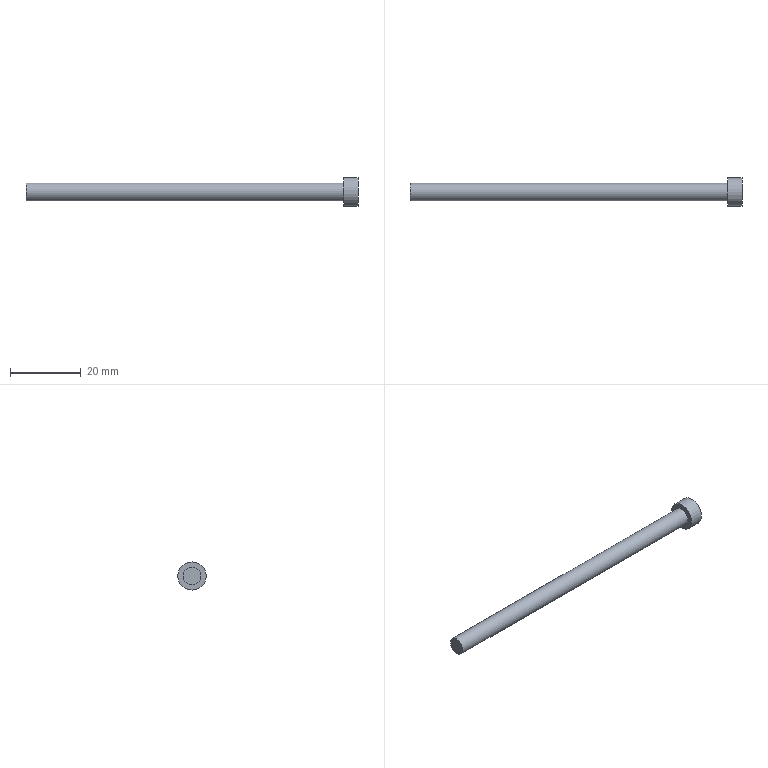Part | STEP file | 1 solid | 5 faces | box 94 x 8 x 8 mm | volume 1968 mm3 | plane 3 | cylinder 2 | commonest cylinder face diameters 5 x1 8 x1
STEP:
#1=CARTESIAN_POINT('',(0.,0.,0.));
#2=DIRECTION('',(0.,0.,1.));
#3=DIRECTION('',(1.,0.,0.));
#4=AXIS2_PLACEMENT_3D('',#1,#2,#3);
#5=CARTESIAN_POINT('',(1660.957,384.98,18.519));
#6=VERTEX_POINT('',#5);
#7=CARTESIAN_POINT('',(1660.957,384.98,16.019));
#8=DIRECTION('',(-1.,0.,0.));
#9=DIRECTION('',(0.,0.,1.));
#10=AXIS2_PLACEMENT_3D('',#7,#8,#9);
#11=CIRCLE('',#10,2.5);
#12=CARTESIAN_POINT('',(1660.957,384.98,16.019));
#13=DIRECTION('',(1.,0.,0.));
#14=DIRECTION('',(0.,0.,-1.));
#15=AXIS2_PLACEMENT_3D('',#12,#13,#14);
#16=CYLINDRICAL_SURFACE('',#15,2.5);
#17=CARTESIAN_POINT('',(9.425,0.));
#18=DIRECTION('',(-1.,0.));
#19=VECTOR('',#18,1.);
#20=LINE('',#17,#19);
#21=(GEOMETRIC_REPRESENTATION_CONTEXT(2)PARAMETRIC_REPRESENTATION_CONTEXT()REPRESENTATION_CONTEXT('',''));
#22=DEFINITIONAL_REPRESENTATION('',(#20),#21);
#23=PCURVE('',#16,#22);
#24=CARTESIAN_POINT('',(1660.957,384.98,16.019));
#25=DIRECTION('',(-1.,0.,0.));
#26=DIRECTION('',(0.,0.,1.));
#27=AXIS2_PLACEMENT_3D('',#24,#25,#26);
#28=PLANE('',#27);
#29=CARTESIAN_POINT('',(0.,0.));
#30=DIRECTION('',(1.,0.));
#31=AXIS2_PLACEMENT_2D('',#29,#30);
#32=CIRCLE('',#31,2.5);
#33=(GEOMETRIC_REPRESENTATION_CONTEXT(2)PARAMETRIC_REPRESENTATION_CONTEXT()REPRESENTATION_CONTEXT('',''));
#34=DEFINITIONAL_REPRESENTATION('',(#32),#33);
#35=PCURVE('',#28,#34);
#36=SURFACE_CURVE('',#11,(#23,#35),.PCURVE_S1.);
#37=EDGE_CURVE('',#6,#6,#36,.T.);
#38=ORIENTED_EDGE('',*,*,#37,.F.);
#39=CARTESIAN_POINT('',(1750.957,384.98,18.519));
#40=VERTEX_POINT('',#39);
#41=CARTESIAN_POINT('',(1660.957,384.98,18.519));
#42=CARTESIAN_POINT('',(1750.957,384.98,18.519));
#43=B_SPLINE_CURVE_WITH_KNOTS('',1,(#41,#42),.UNSPECIFIED.,.F.,.F.,(2,2),(0.,90.),.PIECEWISE_BEZIER_KNOTS.);
#44=CARTESIAN_POINT('',(9.425,0.));
#45=DIRECTION('',(0.,1.));
#46=VECTOR('',#45,1.);
#47=LINE('',#44,#46);
#48=(GEOMETRIC_REPRESENTATION_CONTEXT(2)PARAMETRIC_REPRESENTATION_CONTEXT()REPRESENTATION_CONTEXT('',''));
#49=DEFINITIONAL_REPRESENTATION('',(#47),#48);
#50=PCURVE('',#16,#49);
#51=CARTESIAN_POINT('',(3.142,0.));
#52=DIRECTION('',(0.,1.));
#53=VECTOR('',#52,1.);
#54=LINE('',#51,#53);
#55=(GEOMETRIC_REPRESENTATION_CONTEXT(2)PARAMETRIC_REPRESENTATION_CONTEXT()REPRESENTATION_CONTEXT('',''));
#56=DEFINITIONAL_REPRESENTATION('',(#54),#55);
#57=PCURVE('',#16,#56);
#58=SEAM_CURVE('',#43,(#50,#57),.PCURVE_S1.);
#59=EDGE_CURVE('',#6,#40,#58,.T.);
#60=ORIENTED_EDGE('',*,*,#59,.T.);
#61=CARTESIAN_POINT('',(1750.957,384.98,16.019));
#62=DIRECTION('',(-1.,0.,0.));
#63=DIRECTION('',(0.,0.,1.));
#64=AXIS2_PLACEMENT_3D('',#61,#62,#63);
#65=CIRCLE('',#64,2.5);
#66=CARTESIAN_POINT('',(9.425,90.));
#67=DIRECTION('',(-1.,0.));
#68=VECTOR('',#67,1.);
#69=LINE('',#66,#68);
#70=(GEOMETRIC_REPRESENTATION_CONTEXT(2)PARAMETRIC_REPRESENTATION_CONTEXT()REPRESENTATION_CONTEXT('',''));
#71=DEFINITIONAL_REPRESENTATION('',(#69),#70);
#72=PCURVE('',#16,#71);
#73=CARTESIAN_POINT('',(1750.957,384.98,16.019));
#74=DIRECTION('',(-1.,0.,0.));
#75=DIRECTION('',(0.,0.,1.));
#76=AXIS2_PLACEMENT_3D('',#73,#74,#75);
#77=PLANE('',#76);
#78=CARTESIAN_POINT('',(0.,0.));
#79=DIRECTION('',(1.,0.));
#80=AXIS2_PLACEMENT_2D('',#78,#79);
#81=CIRCLE('',#80,2.5);
#82=(GEOMETRIC_REPRESENTATION_CONTEXT(2)PARAMETRIC_REPRESENTATION_CONTEXT()REPRESENTATION_CONTEXT('',''));
#83=DEFINITIONAL_REPRESENTATION('',(#81),#82);
#84=PCURVE('',#77,#83);
#85=SURFACE_CURVE('',#65,(#72,#84),.PCURVE_S1.);
#86=EDGE_CURVE('',#40,#40,#85,.T.);
#87=ORIENTED_EDGE('',*,*,#86,.T.);
#88=ORIENTED_EDGE('',*,*,#59,.F.);
#89=EDGE_LOOP('',(#38,#60,#87,#88));
#90=FACE_BOUND('',#89,.T.);
#91=ADVANCED_FACE('',(#90),#16,.T.);
#92=ORIENTED_EDGE('',*,*,#37,.T.);
#93=EDGE_LOOP('',(#92));
#94=FACE_BOUND('',#93,.T.);
#95=ADVANCED_FACE('',(#94),#28,.T.);
#96=CARTESIAN_POINT('',(1754.957,384.98,20.019));
#97=VERTEX_POINT('',#96);
#98=CARTESIAN_POINT('',(1754.957,384.98,16.019));
#99=DIRECTION('',(-1.,0.,0.));
#100=DIRECTION('',(0.,0.,1.));
#101=AXIS2_PLACEMENT_3D('',#98,#99,#100);
#102=CIRCLE('',#101,4.);
#103=CARTESIAN_POINT('',(1755.957,384.98,16.019));
#104=DIRECTION('',(-1.,0.,0.));
#105=DIRECTION('',(0.,0.,1.));
#106=AXIS2_PLACEMENT_3D('',#103,#104,#105);
#107=CYLINDRICAL_SURFACE('',#106,4.);
#108=CARTESIAN_POINT('',(0.,1.));
#109=DIRECTION('',(1.,0.));
#110=VECTOR('',#109,1.);
#111=LINE('',#108,#110);
#112=(GEOMETRIC_REPRESENTATION_CONTEXT(2)PARAMETRIC_REPRESENTATION_CONTEXT()REPRESENTATION_CONTEXT('',''));
#113=DEFINITIONAL_REPRESENTATION('',(#111),#112);
#114=PCURVE('',#107,#113);
#115=CARTESIAN_POINT('',(1754.957,384.98,16.019));
#116=DIRECTION('',(-1.,0.,0.));
#117=DIRECTION('',(0.,0.,1.));
#118=AXIS2_PLACEMENT_3D('',#115,#116,#117);
#119=PLANE('',#118);
#120=CARTESIAN_POINT('',(0.,0.));
#121=DIRECTION('',(1.,0.));
#122=AXIS2_PLACEMENT_2D('',#120,#121);
#123=CIRCLE('',#122,4.);
#124=(GEOMETRIC_REPRESENTATION_CONTEXT(2)PARAMETRIC_REPRESENTATION_CONTEXT()REPRESENTATION_CONTEXT('',''));
#125=DEFINITIONAL_REPRESENTATION('',(#123),#124);
#126=PCURVE('',#119,#125);
#127=SURFACE_CURVE('',#102,(#114,#126),.PCURVE_S1.);
#128=EDGE_CURVE('',#97,#97,#127,.T.);
#129=ORIENTED_EDGE('',*,*,#128,.T.);
#130=CARTESIAN_POINT('',(1750.957,384.98,20.019));
#131=VERTEX_POINT('',#130);
#132=CARTESIAN_POINT('',(1754.957,384.98,20.019));
#133=CARTESIAN_POINT('',(1750.957,384.98,20.019));
#134=B_SPLINE_CURVE_WITH_KNOTS('',1,(#132,#133),.UNSPECIFIED.,.F.,.F.,(2,2),(1.,5.),.PIECEWISE_BEZIER_KNOTS.);
#135=CARTESIAN_POINT('',(6.283,0.));
#136=DIRECTION('',(0.,1.));
#137=VECTOR('',#136,1.);
#138=LINE('',#135,#137);
#139=(GEOMETRIC_REPRESENTATION_CONTEXT(2)PARAMETRIC_REPRESENTATION_CONTEXT()REPRESENTATION_CONTEXT('',''));
#140=DEFINITIONAL_REPRESENTATION('',(#138),#139);
#141=PCURVE('',#107,#140);
#142=CARTESIAN_POINT('',(0.,0.));
#143=DIRECTION('',(0.,1.));
#144=VECTOR('',#143,1.);
#145=LINE('',#142,#144);
#146=(GEOMETRIC_REPRESENTATION_CONTEXT(2)PARAMETRIC_REPRESENTATION_CONTEXT()REPRESENTATION_CONTEXT('',''));
#147=DEFINITIONAL_REPRESENTATION('',(#145),#146);
#148=PCURVE('',#107,#147);
#149=SEAM_CURVE('',#134,(#141,#148),.PCURVE_S1.);
#150=EDGE_CURVE('',#97,#131,#149,.T.);
#151=ORIENTED_EDGE('',*,*,#150,.T.);
#152=CARTESIAN_POINT('',(1750.957,384.98,16.019));
#153=DIRECTION('',(-1.,0.,0.));
#154=DIRECTION('',(0.,0.,1.));
#155=AXIS2_PLACEMENT_3D('',#152,#153,#154);
#156=CIRCLE('',#155,4.);
#157=CARTESIAN_POINT('',(0.,5.));
#158=DIRECTION('',(1.,0.));
#159=VECTOR('',#158,1.);
#160=LINE('',#157,#159);
#161=(GEOMETRIC_REPRESENTATION_CONTEXT(2)PARAMETRIC_REPRESENTATION_CONTEXT()REPRESENTATION_CONTEXT('',''));
#162=DEFINITIONAL_REPRESENTATION('',(#160),#161);
#163=PCURVE('',#107,#162);
#164=CARTESIAN_POINT('',(0.,0.));
#165=DIRECTION('',(1.,0.));
#166=AXIS2_PLACEMENT_2D('',#164,#165);
#167=CIRCLE('',#166,4.);
#168=(GEOMETRIC_REPRESENTATION_CONTEXT(2)PARAMETRIC_REPRESENTATION_CONTEXT()REPRESENTATION_CONTEXT('',''));
#169=DEFINITIONAL_REPRESENTATION('',(#167),#168);
#170=PCURVE('',#77,#169);
#171=SURFACE_CURVE('',#156,(#163,#170),.PCURVE_S1.);
#172=EDGE_CURVE('',#131,#131,#171,.T.);
#173=ORIENTED_EDGE('',*,*,#172,.F.);
#174=ORIENTED_EDGE('',*,*,#150,.F.);
#175=EDGE_LOOP('',(#129,#151,#173,#174));
#176=FACE_BOUND('',#175,.T.);
#177=ADVANCED_FACE('',(#176),#107,.T.);
#178=ORIENTED_EDGE('',*,*,#128,.F.);
#179=EDGE_LOOP('',(#178));
#180=FACE_BOUND('',#179,.T.);
#181=ADVANCED_FACE('',(#180),#119,.F.);
#182=ORIENTED_EDGE('',*,*,#86,.F.);
#183=EDGE_LOOP('',(#182));
#184=FACE_BOUND('',#183,.T.);
#185=ORIENTED_EDGE('',*,*,#172,.T.);
#186=EDGE_LOOP('',(#185));
#187=FACE_BOUND('',#186,.T.);
#188=ADVANCED_FACE('',(#184,#187),#77,.T.);
#189=CLOSED_SHELL('',(#91,#95,#177,#181,#188));
#190=MANIFOLD_SOLID_BREP('',#189);
#191=(LENGTH_UNIT()NAMED_UNIT(*)SI_UNIT(.MILLI.,.METRE.));
#192=UNCERTAINTY_MEASURE_WITH_UNIT(LENGTH_MEASURE(0.00001),#191,'','');
#193=(NAMED_UNIT(*)PLANE_ANGLE_UNIT()SI_UNIT($,.RADIAN.));
#194=(NAMED_UNIT(*)SI_UNIT($,.STERADIAN.)SOLID_ANGLE_UNIT());
#195=(GEOMETRIC_REPRESENTATION_CONTEXT(3)GLOBAL_UNCERTAINTY_ASSIGNED_CONTEXT((#192))GLOBAL_UNIT_ASSIGNED_CONTEXT((#191,#193,#194))REPRESENTATION_CONTEXT('',''));
#196=ADVANCED_BREP_SHAPE_REPRESENTATION('',(#4,#190),#195);